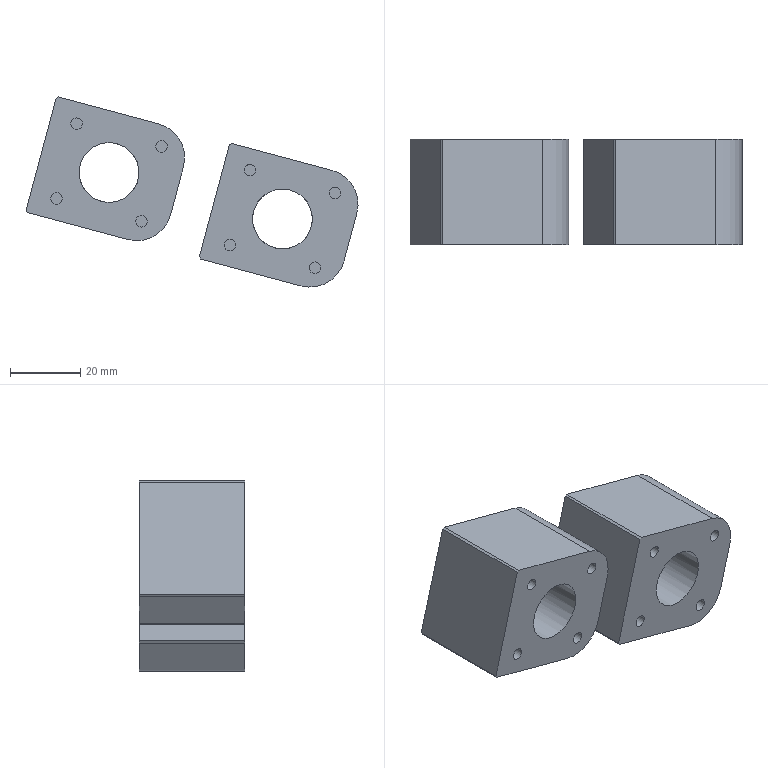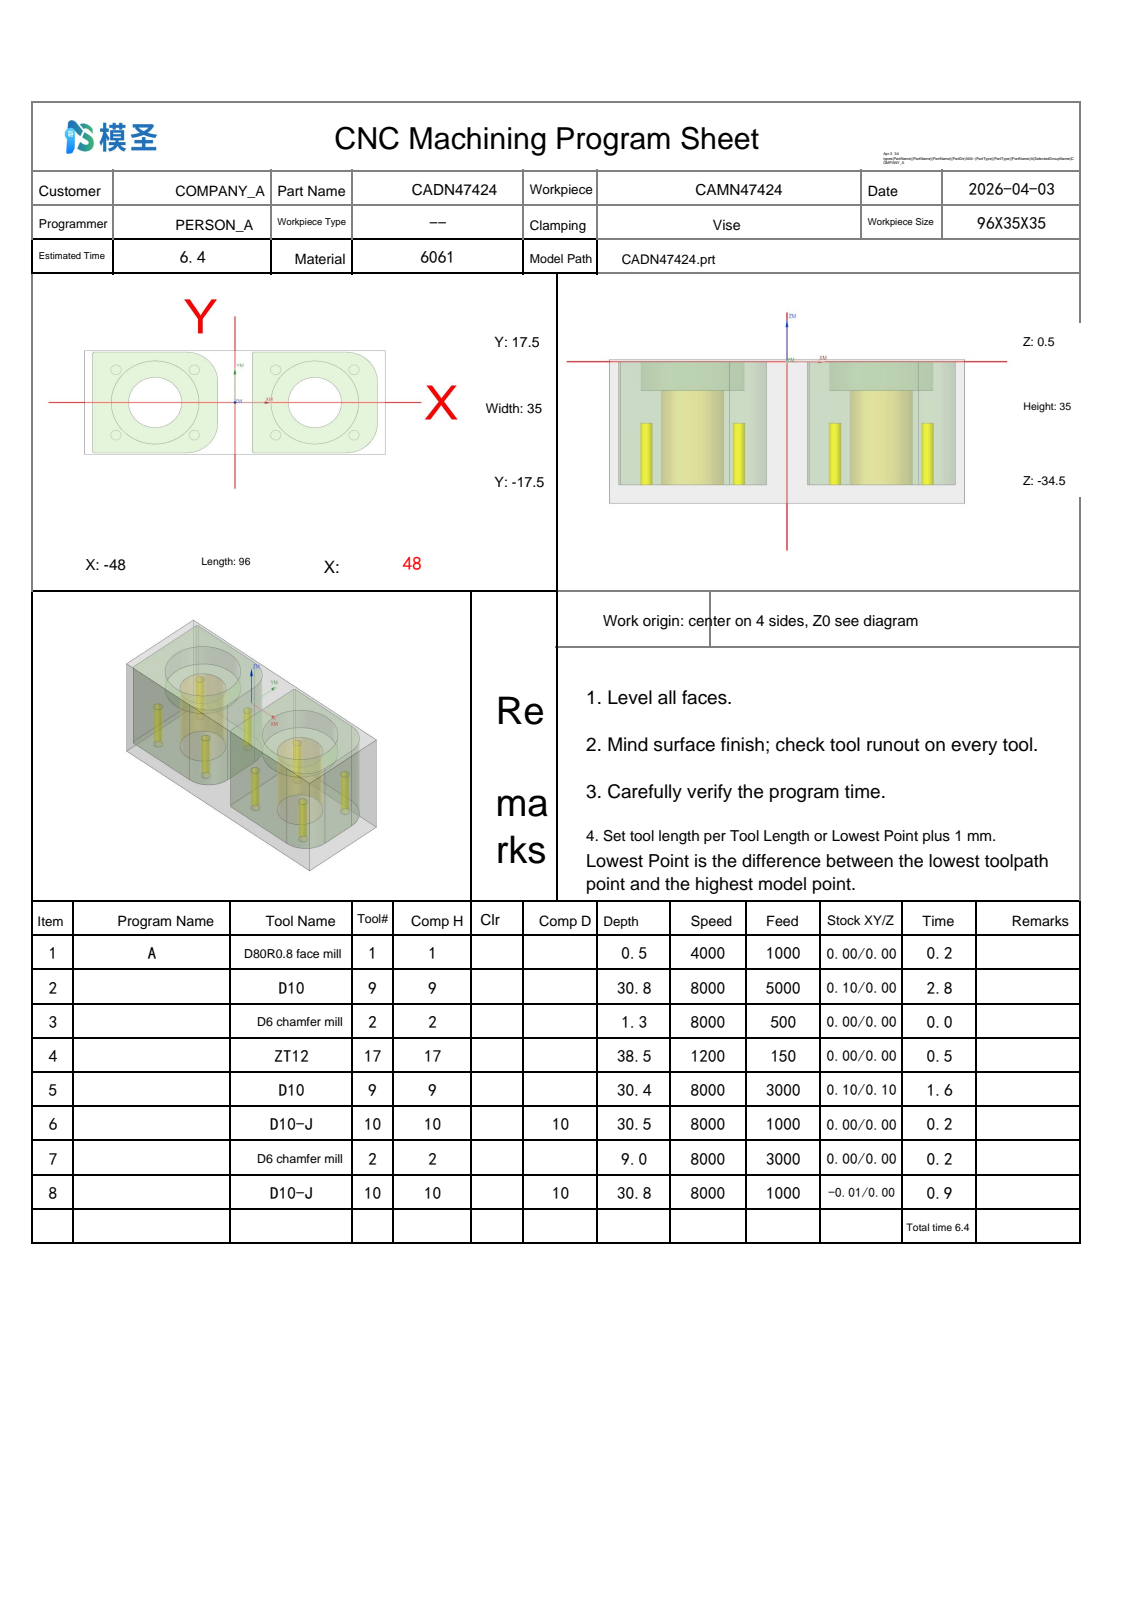NC program | NX | posted by the shop | part box 94.322 x 30 x 54.017 mm
Lines 1043 to 2047 of 2047:
N5 T09 M06
(D10  D=10. R=0. H=09 ce=0.10 di=0.10)
G00 G90 G54 X31.535 Y-6.551 M03 S8000
G43 H09 Z20.
M08
Z1.
G01 X32.075 Y-6.072 Z.962 F3000.
X33.155 Y-4.638 Z.868
X33.927 Y-3.016 Z.774
X34.306 Y-1.601 Z.697
X34.448 Y.189 Z.603
X34.23 Y1.971 Z.509
X33.661 Y3.675 Z.415
X32.763 Y5.23 Z.321
X31.572 Y6.575 Z.227
X30.138 Y7.655 Z.132
X28.516 Y8.427 Z.038
X27.809 Y8.616 Z0.0
G03 X16.884 Y2.309 Z-.123 I-2.309 J-8.616
X23.191 Y-8.616 Z-.246 I8.616 J-2.309
X34.116 Y-2.309 Z-.37 I2.309 J8.616
X27.809 Y8.616 Z-.493 I-8.616 J2.309
X16.884 Y2.309 Z-.616 I-2.309 J-8.616
X23.191 Y-8.616 Z-.739 I8.616 J-2.309
X34.116 Y-2.309 Z-.863 I2.309 J8.616
X27.809 Y8.616 Z-.986 I-8.616 J2.309
X16.884 Y2.309 Z-1.109 I-2.309 J-8.616
X23.191 Y-8.616 Z-1.232 I8.616 J-2.309
X34.116 Y-2.309 Z-1.355 I2.309 J8.616
X27.809 Y8.616 Z-1.479 I-8.616 J2.309
X16.884 Y2.309 Z-1.602 I-2.309 J-8.616
X23.191 Y-8.616 Z-1.725 I8.616 J-2.309
X34.116 Y-2.309 Z-1.848 I2.309 J8.616
X27.809 Y8.616 Z-1.971 I-8.616 J2.309
X16.884 Y2.309 Z-2.095 I-2.309 J-8.616
X23.191 Y-8.616 Z-2.218 I8.616 J-2.309
X34.116 Y-2.309 Z-2.341 I2.309 J8.616
X27.809 Y8.616 Z-2.464 I-8.616 J2.309
X16.884 Y2.309 Z-2.588 I-2.309 J-8.616
X23.191 Y-8.616 Z-2.711 I8.616 J-2.309
X34.116 Y-2.309 Z-2.834 I2.309 J8.616
X27.809 Y8.616 Z-2.957 I-8.616 J2.309
X16.884 Y2.309 Z-3.08 I-2.309 J-8.616
X23.191 Y-8.616 Z-3.204 I8.616 J-2.309
X34.116 Y-2.309 Z-3.327 I2.309 J8.616
X27.809 Y8.616 Z-3.45 I-8.616 J2.309
X16.884 Y2.309 Z-3.573 I-2.309 J-8.616
X23.191 Y-8.616 Z-3.696 I8.616 J-2.309
X34.116 Y-2.309 Z-3.82 I2.309 J8.616
X27.809 Y8.616 Z-3.943 I-8.616 J2.309
X16.884 Y2.309 Z-4.066 I-2.309 J-8.616
X23.191 Y-8.616 Z-4.189 I8.616 J-2.309
X34.116 Y-2.309 Z-4.313 I2.309 J8.616
X27.809 Y8.616 Z-4.436 I-8.616 J2.309
X16.884 Y2.309 Z-4.559 I-2.309 J-8.616
X23.191 Y-8.616 Z-4.682 I8.616 J-2.309
X34.116 Y-2.309 Z-4.805 I2.309 J8.616
X27.809 Y8.616 Z-4.929 I-8.616 J2.309
X16.884 Y2.309 Z-5.052 I-2.309 J-8.616
X23.191 Y-8.616 Z-5.175 I8.616 J-2.309
X34.116 Y-2.309 Z-5.298 I2.309 J8.616
X27.809 Y8.616 Z-5.421 I-8.616 J2.309
X16.884 Y2.309 Z-5.545 I-2.309 J-8.616
X23.191 Y-8.616 Z-5.668 I8.616 J-2.309
X34.116 Y-2.309 Z-5.791 I2.309 J8.616
X27.809 Y8.616 Z-5.914 I-8.616 J2.309
X16.884 Y2.309 Z-6.038 I-2.309 J-8.616
X23.191 Y-8.616 Z-6.161 I8.616 J-2.309
X34.116 Y-2.309 Z-6.284 I2.309 J8.616
X27.809 Y8.616 Z-6.407 I-8.616 J2.309
X16.884 Y2.309 Z-6.53 I-2.309 J-8.616
X23.191 Y-8.616 Z-6.654 I8.616 J-2.309
X34.116 Y-2.309 Z-6.777 I2.309 J8.616
X27.809 Y8.616 Z-6.9 I-8.616 J2.309
X25.5 Y8.92 I-2.309 J-8.616
X16.58 Y0.0 I0.0 J-8.92
X25.5 Y-8.92 I8.92 J0.0
X34.42 Y0.0 I0.0 J8.92
X27.809 Y8.616 I-8.92 J0.0
X27.42 Y8.711 I-2.309 J-8.616
G01 Z-5.9
G00 Z20.
X-31.535 Y6.551
Z1.
G01 X-32.075 Y6.072 Z.962
X-33.155 Y4.638 Z.868
X-33.927 Y3.016 Z.774
X-34.306 Y1.601 Z.697
X-34.448 Y-.189 Z.603
X-34.23 Y-1.971 Z.509
X-33.661 Y-3.675 Z.415
X-32.763 Y-5.23 Z.321
X-31.572 Y-6.575 Z.227
X-30.138 Y-7.655 Z.132
X-28.516 Y-8.427 Z.038
X-27.809 Y-8.616 Z0.0
G03 X-16.884 Y-2.309 Z-.123 I2.309 J8.616
X-18.483 Y5.508 Z-.196 I-8.616 J2.309
X-23.191 Y8.616 Z-.246 I-7.017 J-5.508
X-34.116 Y2.309 Z-.37 I-2.309 J-8.616
X-27.809 Y-8.616 Z-.493 I8.616 J-2.309
X-16.884 Y-2.309 Z-.616 I2.309 J8.616
X-18.483 Y5.508 Z-.689 I-8.616 J2.309
X-23.191 Y8.616 Z-.739 I-7.017 J-5.508
X-34.116 Y2.309 Z-.863 I-2.309 J-8.616
X-27.809 Y-8.616 Z-.986 I8.616 J-2.309
X-16.884 Y-2.309 Z-1.109 I2.309 J8.616
X-18.483 Y5.508 Z-1.182 I-8.616 J2.309
X-23.191 Y8.616 Z-1.232 I-7.017 J-5.508
X-34.116 Y2.309 Z-1.355 I-2.309 J-8.616
X-27.809 Y-8.616 Z-1.479 I8.616 J-2.309
X-16.884 Y-2.309 Z-1.602 I2.309 J8.616
X-18.483 Y5.508 Z-1.675 I-8.616 J2.309
X-23.191 Y8.616 Z-1.725 I-7.017 J-5.508
X-34.116 Y2.309 Z-1.848 I-2.309 J-8.616
X-27.809 Y-8.616 Z-1.971 I8.616 J-2.309
X-16.884 Y-2.309 Z-2.095 I2.309 J8.616
X-18.483 Y5.508 Z-2.167 I-8.616 J2.309
X-23.191 Y8.616 Z-2.218 I-7.017 J-5.508
X-34.116 Y2.309 Z-2.341 I-2.309 J-8.616
X-27.809 Y-8.616 Z-2.464 I8.616 J-2.309
X-16.884 Y-2.309 Z-2.588 I2.309 J8.616
X-18.483 Y5.508 Z-2.66 I-8.616 J2.309
X-23.191 Y8.616 Z-2.711 I-7.017 J-5.508
X-34.116 Y2.309 Z-2.834 I-2.309 J-8.616
X-27.809 Y-8.616 Z-2.957 I8.616 J-2.309
X-16.884 Y-2.309 Z-3.08 I2.309 J8.616
X-18.483 Y5.508 Z-3.153 I-8.616 J2.309
X-23.191 Y8.616 Z-3.204 I-7.017 J-5.508
X-34.116 Y2.309 Z-3.327 I-2.309 J-8.616
X-27.809 Y-8.616 Z-3.45 I8.616 J-2.309
X-16.884 Y-2.309 Z-3.573 I2.309 J8.616
X-18.483 Y5.508 Z-3.646 I-8.616 J2.309
X-23.191 Y8.616 Z-3.696 I-7.017 J-5.508
X-34.116 Y2.309 Z-3.82 I-2.309 J-8.616
X-27.809 Y-8.616 Z-3.943 I8.616 J-2.309
X-16.884 Y-2.309 Z-4.066 I2.309 J8.616
X-18.483 Y5.508 Z-4.139 I-8.616 J2.309
X-23.191 Y8.616 Z-4.189 I-7.017 J-5.508
X-34.116 Y2.309 Z-4.313 I-2.309 J-8.616
X-27.809 Y-8.616 Z-4.436 I8.616 J-2.309
X-16.884 Y-2.309 Z-4.559 I2.309 J8.616
X-18.483 Y5.508 Z-4.632 I-8.616 J2.309
X-23.191 Y8.616 Z-4.682 I-7.017 J-5.508
X-34.116 Y2.309 Z-4.805 I-2.309 J-8.616
X-27.809 Y-8.616 Z-4.929 I8.616 J-2.309
X-16.884 Y-2.309 Z-5.052 I2.309 J8.616
X-18.483 Y5.508 Z-5.125 I-8.616 J2.309
X-23.191 Y8.616 Z-5.175 I-7.017 J-5.508
X-34.116 Y2.309 Z-5.298 I-2.309 J-8.616
X-27.809 Y-8.616 Z-5.421 I8.616 J-2.309
X-16.884 Y-2.309 Z-5.545 I2.309 J8.616
X-18.483 Y5.508 Z-5.617 I-8.616 J2.309
X-23.191 Y8.616 Z-5.668 I-7.017 J-5.508
X-34.116 Y2.309 Z-5.791 I-2.309 J-8.616
X-27.809 Y-8.616 Z-5.914 I8.616 J-2.309
X-16.884 Y-2.309 Z-6.038 I2.309 J8.616
X-18.483 Y5.508 Z-6.11 I-8.616 J2.309
X-23.191 Y8.616 Z-6.161 I-7.017 J-5.508
X-34.116 Y2.309 Z-6.284 I-2.309 J-8.616
X-27.809 Y-8.616 Z-6.407 I8.616 J-2.309
X-16.884 Y-2.309 Z-6.53 I2.309 J8.616
X-18.483 Y5.508 Z-6.603 I-8.616 J2.309
X-23.191 Y8.616 Z-6.654 I-7.017 J-5.508
X-34.116 Y2.309 Z-6.777 I-2.309 J-8.616
X-27.809 Y-8.616 Z-6.9 I8.616 J-2.309
X-25.5 Y-8.92 I2.309 J8.616
X-16.58 Y0.0 I0.0 J8.92
X-25.5 Y8.92 I-8.92 J0.0
X-34.42 Y0.0 I0.0 J-8.92
X-27.809 Y-8.616 I8.92 J0.0
X-27.42 Y-8.711 I2.309 J8.616
G01 Z-5.9
G00 Z20.
G00 G90 X24.068 Y3.077 M03 S8000
Z20.
Z-6.
G01 X23.785 Y2.97 Z-6.016 F2000.
X22.923 Y2.263 Z-6.074
X22.333 Y1.317 Z-6.133
X22.099 Y.443 Z-6.18
X22.136 Y-.672 Z-6.239
X22.53 Y-1.715 Z-6.297
X23.237 Y-2.577 Z-6.355
X24.183 Y-3.167 Z-6.414
X25.057 Y-3.401 Z-6.461
X26.172 Y-3.364 Z-6.52
X27.215 Y-2.97 Z-6.578
X28.077 Y-2.263 Z-6.637
X28.667 Y-1.317 Z-6.695
X28.901 Y-.443 Z-6.743
X28.864 Y.672 Z-6.801
X28.47 Y1.715 Z-6.859
X27.763 Y2.577 Z-6.918
X26.817 Y3.167 Z-6.976
X26.38 Y3.284 Z-7.
G03 X22.216 Y.88 Z-7.124 I-.88 J-3.284
X24.62 Y-3.284 Z-7.249 I3.284 J-.88
X28.784 Y-.88 Z-7.373 I.88 J3.284
X26.38 Y3.284 Z-7.498 I-3.284 J.88
X22.216 Y.88 Z-7.622 I-.88 J-3.284
X24.62 Y-3.284 Z-7.747 I3.284 J-.88
X28.784 Y-.88 Z-7.871 I.88 J3.284
X26.38 Y3.284 Z-7.996 I-3.284 J.88
X22.216 Y.88 Z-8.12 I-.88 J-3.284
X24.62 Y-3.284 Z-8.245 I3.284 J-.88
X28.784 Y-.88 Z-8.369 I.88 J3.284
X26.38 Y3.284 Z-8.493 I-3.284 J.88
X22.216 Y.88 Z-8.618 I-.88 J-3.284
X24.62 Y-3.284 Z-8.742 I3.284 J-.88
X28.784 Y-.88 Z-8.867 I.88 J3.284
X26.38 Y3.284 Z-8.991 I-3.284 J.88
X22.216 Y.88 Z-9.116 I-.88 J-3.284
X24.62 Y-3.284 Z-9.24 I3.284 J-.88
X28.784 Y-.88 Z-9.365 I.88 J3.284
X26.38 Y3.284 Z-9.489 I-3.284 J.88
X22.216 Y.88 Z-9.614 I-.88 J-3.284
X24.62 Y-3.284 Z-9.738 I3.284 J-.88
X28.784 Y-.88 Z-9.863 I.88 J3.284
X26.38 Y3.284 Z-9.987 I-3.284 J.88
X22.216 Y.88 Z-10.111 I-.88 J-3.284
X24.62 Y-3.284 Z-10.236 I3.284 J-.88
X28.784 Y-.88 Z-10.36 I.88 J3.284
X26.38 Y3.284 Z-10.485 I-3.284 J.88
X22.216 Y.88 Z-10.609 I-.88 J-3.284
X24.62 Y-3.284 Z-10.734 I3.284 J-.88
X28.784 Y-.88 Z-10.858 I.88 J3.284
X26.38 Y3.284 Z-10.983 I-3.284 J.88
X22.216 Y.88 Z-11.107 I-.88 J-3.284
X24.62 Y-3.284 Z-11.232 I3.284 J-.88
X28.784 Y-.88 Z-11.356 I.88 J3.284
X26.38 Y3.284 Z-11.48 I-3.284 J.88
X22.216 Y.88 Z-11.605 I-.88 J-3.284
X24.62 Y-3.284 Z-11.729 I3.284 J-.88
X28.784 Y-.88 Z-11.854 I.88 J3.284
X26.38 Y3.284 Z-11.978 I-3.284 J.88
X22.216 Y.88 Z-12.103 I-.88 J-3.284
X24.62 Y-3.284 Z-12.227 I3.284 J-.88
X28.784 Y-.88 Z-12.352 I.88 J3.284
X26.38 Y3.284 Z-12.476 I-3.284 J.88
X22.216 Y.88 Z-12.601 I-.88 J-3.284
X24.62 Y-3.284 Z-12.725 I3.284 J-.88
X28.784 Y-.88 Z-12.849 I.88 J3.284
X26.38 Y3.284 Z-12.974 I-3.284 J.88
X22.216 Y.88 Z-13.098 I-.88 J-3.284
X24.62 Y-3.284 Z-13.223 I3.284 J-.88
X28.784 Y-.88 Z-13.347 I.88 J3.284
X26.38 Y3.284 Z-13.472 I-3.284 J.88
X22.216 Y.88 Z-13.596 I-.88 J-3.284
X24.62 Y-3.284 Z-13.721 I3.284 J-.88
X28.784 Y-.88 Z-13.845 I.88 J3.284
X26.38 Y3.284 Z-13.97 I-3.284 J.88
X22.216 Y.88 Z-14.094 I-.88 J-3.284
X24.62 Y-3.284 Z-14.218 I3.284 J-.88
X28.784 Y-.88 Z-14.343 I.88 J3.284
X26.38 Y3.284 Z-14.467 I-3.284 J.88
X22.216 Y.88 Z-14.592 I-.88 J-3.284
X24.62 Y-3.284 Z-14.716 I3.284 J-.88
X28.784 Y-.88 Z-14.841 I.88 J3.284
X26.38 Y3.284 Z-14.965 I-3.284 J.88
X22.216 Y.88 Z-15.09 I-.88 J-3.284
X24.62 Y-3.284 Z-15.214 I3.284 J-.88
X28.784 Y-.88 Z-15.339 I.88 J3.284
X26.38 Y3.284 Z-15.463 I-3.284 J.88
X22.216 Y.88 Z-15.588 I-.88 J-3.284
X24.62 Y-3.284 Z-15.712 I3.284 J-.88
X28.784 Y-.88 Z-15.836 I.88 J3.284
X26.38 Y3.284 Z-15.961 I-3.284 J.88
X22.216 Y.88 Z-16.085 I-.88 J-3.284
X24.62 Y-3.284 Z-16.21 I3.284 J-.88
X28.784 Y-.88 Z-16.334 I.88 J3.284
X26.38 Y3.284 Z-16.459 I-3.284 J.88
X22.216 Y.88 Z-16.583 I-.88 J-3.284
X24.62 Y-3.284 Z-16.708 I3.284 J-.88
X28.784 Y-.88 Z-16.832 I.88 J3.284
X26.38 Y3.284 Z-16.957 I-3.284 J.88
X22.216 Y.88 Z-17.081 I-.88 J-3.284
X24.62 Y-3.284 Z-17.205 I3.284 J-.88
X28.784 Y-.88 Z-17.33 I.88 J3.284
X26.38 Y3.284 Z-17.454 I-3.284 J.88
X22.216 Y.88 Z-17.579 I-.88 J-3.284
X24.62 Y-3.284 Z-17.703 I3.284 J-.88
X28.784 Y-.88 Z-17.828 I.88 J3.284
X26.38 Y3.284 Z-17.952 I-3.284 J.88
X22.216 Y.88 Z-18.077 I-.88 J-3.284
X24.62 Y-3.284 Z-18.201 I3.284 J-.88
X28.784 Y-.88 Z-18.326 I.88 J3.284
X26.38 Y3.284 Z-18.45 I-3.284 J.88
X22.216 Y.88 Z-18.574 I-.88 J-3.284
X24.62 Y-3.284 Z-18.699 I3.284 J-.88
X28.784 Y-.88 Z-18.823 I.88 J3.284
X26.38 Y3.284 Z-18.948 I-3.284 J.88
X22.216 Y.88 Z-19.072 I-.88 J-3.284
X24.62 Y-3.284 Z-19.197 I3.284 J-.88
X28.784 Y-.88 Z-19.321 I.88 J3.284
X26.38 Y3.284 Z-19.446 I-3.284 J.88
X22.216 Y.88 Z-19.57 I-.88 J-3.284
X24.62 Y-3.284 Z-19.695 I3.284 J-.88
X28.784 Y-.88 Z-19.819 I.88 J3.284
X26.38 Y3.284 Z-19.943 I-3.284 J.88
X22.216 Y.88 Z-20.068 I-.88 J-3.284
X24.62 Y-3.284 Z-20.192 I3.284 J-.88
X28.784 Y-.88 Z-20.317 I.88 J3.284
X26.38 Y3.284 Z-20.441 I-3.284 J.88
X22.216 Y.88 Z-20.566 I-.88 J-3.284
X24.62 Y-3.284 Z-20.69 I3.284 J-.88
X28.784 Y-.88 Z-20.815 I.88 J3.284
X26.38 Y3.284 Z-20.939 I-3.284 J.88
X22.216 Y.88 Z-21.064 I-.88 J-3.284
X24.62 Y-3.284 Z-21.188 I3.284 J-.88
X28.784 Y-.88 Z-21.313 I.88 J3.284
X26.38 Y3.284 Z-21.437 I-3.284 J.88
X22.216 Y.88 Z-21.561 I-.88 J-3.284
X24.62 Y-3.284 Z-21.686 I3.284 J-.88
X28.784 Y-.88 Z-21.81 I.88 J3.284
X26.38 Y3.284 Z-21.935 I-3.284 J.88
X22.216 Y.88 Z-22.059 I-.88 J-3.284
X24.62 Y-3.284 Z-22.184 I3.284 J-.88
X28.784 Y-.88 Z-22.308 I.88 J3.284
X26.38 Y3.284 Z-22.433 I-3.284 J.88
X22.216 Y.88 Z-22.557 I-.88 J-3.284
X24.62 Y-3.284 Z-22.682 I3.284 J-.88
X28.784 Y-.88 Z-22.806 I.88 J3.284
X26.38 Y3.284 Z-22.93 I-3.284 J.88
X22.216 Y.88 Z-23.055 I-.88 J-3.284
X24.62 Y-3.284 Z-23.179 I3.284 J-.88
X28.784 Y-.88 Z-23.304 I.88 J3.284
X26.38 Y3.284 Z-23.428 I-3.284 J.88
X22.216 Y.88 Z-23.553 I-.88 J-3.284
X24.62 Y-3.284 Z-23.677 I3.284 J-.88
X28.784 Y-.88 Z-23.802 I.88 J3.284
X26.38 Y3.284 Z-23.926 I-3.284 J.88
X22.216 Y.88 Z-24.051 I-.88 J-3.284
X24.62 Y-3.284 Z-24.175 I3.284 J-.88
X28.784 Y-.88 Z-24.299 I.88 J3.284
X26.38 Y3.284 Z-24.424 I-3.284 J.88
X22.216 Y.88 Z-24.548 I-.88 J-3.284
X24.62 Y-3.284 Z-24.673 I3.284 J-.88
X28.784 Y-.88 Z-24.797 I.88 J3.284
X26.38 Y3.284 Z-24.922 I-3.284 J.88
X22.216 Y.88 Z-25.046 I-.88 J-3.284
X24.62 Y-3.284 Z-25.171 I3.284 J-.88
X28.784 Y-.88 Z-25.295 I.88 J3.284
X26.38 Y3.284 Z-25.42 I-3.284 J.88
X22.216 Y.88 Z-25.544 I-.88 J-3.284
X24.62 Y-3.284 Z-25.668 I3.284 J-.88
X28.784 Y-.88 Z-25.793 I.88 J3.284
X26.38 Y3.284 Z-25.917 I-3.284 J.88
X22.216 Y.88 Z-26.042 I-.88 J-3.284
X24.62 Y-3.284 Z-26.166 I3.284 J-.88
X28.784 Y-.88 Z-26.291 I.88 J3.284
X26.38 Y3.284 Z-26.415 I-3.284 J.88
X22.216 Y.88 Z-26.54 I-.88 J-3.284
X24.62 Y-3.284 Z-26.664 I3.284 J-.88
X28.784 Y-.88 Z-26.789 I.88 J3.284
X26.38 Y3.284 Z-26.913 I-3.284 J.88
X22.216 Y.88 Z-27.038 I-.88 J-3.284
X24.62 Y-3.284 Z-27.162 I3.284 J-.88
X28.784 Y-.88 Z-27.286 I.88 J3.284
X26.38 Y3.284 Z-27.411 I-3.284 J.88
X22.216 Y.88 Z-27.535 I-.88 J-3.284
X24.62 Y-3.284 Z-27.66 I3.284 J-.88
X28.784 Y-.88 Z-27.784 I.88 J3.284
X26.38 Y3.284 Z-27.909 I-3.284 J.88
X22.216 Y.88 Z-28.033 I-.88 J-3.284
X24.62 Y-3.284 Z-28.158 I3.284 J-.88
X28.784 Y-.88 Z-28.282 I.88 J3.284
X26.38 Y3.284 Z-28.407 I-3.284 J.88
X22.216 Y.88 Z-28.531 I-.88 J-3.284
X24.62 Y-3.284 Z-28.655 I3.284 J-.88
X28.784 Y-.88 Z-28.78 I.88 J3.284
X26.38 Y3.284 Z-28.904 I-3.284 J.88
X22.216 Y.88 Z-29.029 I-.88 J-3.284
X24.62 Y-3.284 Z-29.153 I3.284 J-.88
X28.784 Y-.88 Z-29.278 I.88 J3.284
X26.38 Y3.284 Z-29.402 I-3.284 J.88
X22.216 Y.88 Z-29.527 I-.88 J-3.284
X24.62 Y-3.284 Z-29.651 I3.284 J-.88
X28.784 Y-.88 Z-29.776 I.88 J3.284
X26.38 Y3.284 Z-29.9 I-3.284 J.88
X25.5 Y3.4 I-.88 J-3.284
X22.1 Y0.0 I0.0 J-3.4
X25.5 Y-3.4 I3.4 J0.0
X28.9 Y0.0 I0.0 J3.4
X26.38 Y3.284 I-3.4 J0.0
X25.988 Y3.365 I-.88 J-3.284
G01 Z-28.9
G00 Z20.
X-24.068 Y-3.077
Z-6.
G01 X-23.785 Y-2.97 Z-6.016
X-22.923 Y-2.263 Z-6.074
X-22.333 Y-1.317 Z-6.133
X-22.099 Y-.443 Z-6.18
X-22.136 Y.672 Z-6.239
X-22.53 Y1.715 Z-6.297
X-23.237 Y2.577 Z-6.355
X-24.183 Y3.167 Z-6.414
X-25.057 Y3.401 Z-6.461
X-26.172 Y3.364 Z-6.52
X-27.215 Y2.97 Z-6.578
X-28.077 Y2.263 Z-6.637
X-28.667 Y1.317 Z-6.695
X-28.901 Y.443 Z-6.743
X-28.864 Y-.672 Z-6.801
X-28.47 Y-1.715 Z-6.859
X-27.763 Y-2.577 Z-6.918
X-26.817 Y-3.167 Z-6.976
X-26.38 Y-3.284 Z-7.
G03 X-22.216 Y-.88 Z-7.124 I.88 J3.284
X-24.62 Y3.284 Z-7.249 I-3.284 J.88
X-28.784 Y.88 Z-7.373 I-.88 J-3.284
X-26.38 Y-3.284 Z-7.498 I3.284 J-.88
X-22.216 Y-.88 Z-7.622 I.88 J3.284
X-24.62 Y3.284 Z-7.747 I-3.284 J.88
X-28.784 Y.88 Z-7.871 I-.88 J-3.284
X-26.38 Y-3.284 Z-7.996 I3.284 J-.88
X-22.216 Y-.88 Z-8.12 I.88 J3.284
X-24.62 Y3.284 Z-8.245 I-3.284 J.88
X-28.784 Y.88 Z-8.369 I-.88 J-3.284
X-26.38 Y-3.284 Z-8.493 I3.284 J-.88
X-22.216 Y-.88 Z-8.618 I.88 J3.284
X-24.62 Y3.284 Z-8.742 I-3.284 J.88
X-28.784 Y.88 Z-8.867 I-.88 J-3.284
X-26.38 Y-3.284 Z-8.991 I3.284 J-.88
X-22.216 Y-.88 Z-9.116 I.88 J3.284
X-24.62 Y3.284 Z-9.24 I-3.284 J.88
X-28.784 Y.88 Z-9.365 I-.88 J-3.284
X-26.38 Y-3.284 Z-9.489 I3.284 J-.88
X-22.216 Y-.88 Z-9.614 I.88 J3.284
X-24.62 Y3.284 Z-9.738 I-3.284 J.88
X-28.784 Y.88 Z-9.863 I-.88 J-3.284
X-26.38 Y-3.284 Z-9.987 I3.284 J-.88
X-22.216 Y-.88 Z-10.111 I.88 J3.284
X-24.62 Y3.284 Z-10.236 I-3.284 J.88
X-28.784 Y.88 Z-10.36 I-.88 J-3.284
X-26.38 Y-3.284 Z-10.485 I3.284 J-.88
X-22.216 Y-.88 Z-10.609 I.88 J3.284
X-24.62 Y3.284 Z-10.734 I-3.284 J.88
X-28.784 Y.88 Z-10.858 I-.88 J-3.284
X-26.38 Y-3.284 Z-10.983 I3.284 J-.88
X-22.216 Y-.88 Z-11.107 I.88 J3.284
X-24.62 Y3.284 Z-11.232 I-3.284 J.88
X-28.784 Y.88 Z-11.356 I-.88 J-3.284
X-26.38 Y-3.284 Z-11.48 I3.284 J-.88
X-22.216 Y-.88 Z-11.605 I.88 J3.284
X-24.62 Y3.284 Z-11.729 I-3.284 J.88
X-28.784 Y.88 Z-11.854 I-.88 J-3.284
X-26.38 Y-3.284 Z-11.978 I3.284 J-.88
X-22.216 Y-.88 Z-12.103 I.88 J3.284
X-24.62 Y3.284 Z-12.227 I-3.284 J.88
X-28.784 Y.88 Z-12.352 I-.88 J-3.284
X-26.38 Y-3.284 Z-12.476 I3.284 J-.88
X-22.216 Y-.88 Z-12.601 I.88 J3.284
X-24.62 Y3.284 Z-12.725 I-3.284 J.88
X-28.784 Y.88 Z-12.849 I-.88 J-3.284
X-26.38 Y-3.284 Z-12.974 I3.284 J-.88
X-22.216 Y-.88 Z-13.098 I.88 J3.284
X-24.62 Y3.284 Z-13.223 I-3.284 J.88
X-28.784 Y.88 Z-13.347 I-.88 J-3.284
X-26.38 Y-3.284 Z-13.472 I3.284 J-.88
X-22.216 Y-.88 Z-13.596 I.88 J3.284
X-24.62 Y3.284 Z-13.721 I-3.284 J.88
X-28.784 Y.88 Z-13.845 I-.88 J-3.284
X-26.38 Y-3.284 Z-13.97 I3.284 J-.88
X-22.216 Y-.88 Z-14.094 I.88 J3.284
X-24.62 Y3.284 Z-14.218 I-3.284 J.88
X-28.784 Y.88 Z-14.343 I-.88 J-3.284
X-26.38 Y-3.284 Z-14.467 I3.284 J-.88
X-22.216 Y-.88 Z-14.592 I.88 J3.284
X-24.62 Y3.284 Z-14.716 I-3.284 J.88
X-28.784 Y.88 Z-14.841 I-.88 J-3.284
X-26.38 Y-3.284 Z-14.965 I3.284 J-.88
X-22.216 Y-.88 Z-15.09 I.88 J3.284
X-24.62 Y3.284 Z-15.214 I-3.284 J.88
X-28.784 Y.88 Z-15.339 I-.88 J-3.284
X-26.38 Y-3.284 Z-15.463 I3.284 J-.88
X-22.216 Y-.88 Z-15.588 I.88 J3.284
X-24.62 Y3.284 Z-15.712 I-3.284 J.88
X-28.784 Y.88 Z-15.836 I-.88 J-3.284
X-26.38 Y-3.284 Z-15.961 I3.284 J-.88
X-22.216 Y-.88 Z-16.085 I.88 J3.284
X-24.62 Y3.284 Z-16.21 I-3.284 J.88
X-28.784 Y.88 Z-16.334 I-.88 J-3.284
X-26.38 Y-3.284 Z-16.459 I3.284 J-.88
X-22.216 Y-.88 Z-16.583 I.88 J3.284
X-24.62 Y3.284 Z-16.708 I-3.284 J.88
X-28.784 Y.88 Z-16.832 I-.88 J-3.284
X-26.38 Y-3.284 Z-16.957 I3.284 J-.88
X-22.216 Y-.88 Z-17.081 I.88 J3.284
X-24.62 Y3.284 Z-17.205 I-3.284 J.88
X-28.784 Y.88 Z-17.33 I-.88 J-3.284
X-26.38 Y-3.284 Z-17.454 I3.284 J-.88
X-22.216 Y-.88 Z-17.579 I.88 J3.284
X-24.62 Y3.284 Z-17.703 I-3.284 J.88
X-28.784 Y.88 Z-17.828 I-.88 J-3.284
X-26.38 Y-3.284 Z-17.952 I3.284 J-.88
X-22.216 Y-.88 Z-18.077 I.88 J3.284
X-24.62 Y3.284 Z-18.201 I-3.284 J.88
X-28.784 Y.88 Z-18.326 I-.88 J-3.284
X-26.38 Y-3.284 Z-18.45 I3.284 J-.88
X-22.216 Y-.88 Z-18.574 I.88 J3.284
X-24.62 Y3.284 Z-18.699 I-3.284 J.88
X-28.784 Y.88 Z-18.823 I-.88 J-3.284
X-26.38 Y-3.284 Z-18.948 I3.284 J-.88
X-22.216 Y-.88 Z-19.072 I.88 J3.284
X-24.62 Y3.284 Z-19.197 I-3.284 J.88
X-28.784 Y.88 Z-19.321 I-.88 J-3.284
X-26.38 Y-3.284 Z-19.446 I3.284 J-.88
X-22.216 Y-.88 Z-19.57 I.88 J3.284
X-24.62 Y3.284 Z-19.695 I-3.284 J.88
X-28.784 Y.88 Z-19.819 I-.88 J-3.284
X-26.38 Y-3.284 Z-19.943 I3.284 J-.88
X-22.216 Y-.88 Z-20.068 I.88 J3.284
X-24.62 Y3.284 Z-20.192 I-3.284 J.88
X-28.784 Y.88 Z-20.317 I-.88 J-3.284
X-26.38 Y-3.284 Z-20.441 I3.284 J-.88
X-22.216 Y-.88 Z-20.566 I.88 J3.284
X-24.62 Y3.284 Z-20.69 I-3.284 J.88
X-28.784 Y.88 Z-20.815 I-.88 J-3.284
X-26.38 Y-3.284 Z-20.939 I3.284 J-.88
X-22.216 Y-.88 Z-21.064 I.88 J3.284
X-24.62 Y3.284 Z-21.188 I-3.284 J.88
X-28.784 Y.88 Z-21.313 I-.88 J-3.284
X-26.38 Y-3.284 Z-21.437 I3.284 J-.88
X-22.216 Y-.88 Z-21.561 I.88 J3.284
X-24.62 Y3.284 Z-21.686 I-3.284 J.88
X-28.784 Y.88 Z-21.81 I-.88 J-3.284
X-26.38 Y-3.284 Z-21.935 I3.284 J-.88
X-22.216 Y-.88 Z-22.059 I.88 J3.284
X-24.62 Y3.284 Z-22.184 I-3.284 J.88
X-28.784 Y.88 Z-22.308 I-.88 J-3.284
X-26.38 Y-3.284 Z-22.433 I3.284 J-.88
X-22.216 Y-.88 Z-22.557 I.88 J3.284
X-24.62 Y3.284 Z-22.682 I-3.284 J.88
X-28.784 Y.88 Z-22.806 I-.88 J-3.284
X-26.38 Y-3.284 Z-22.93 I3.284 J-.88
X-22.216 Y-.88 Z-23.055 I.88 J3.284
X-24.62 Y3.284 Z-23.179 I-3.284 J.88
X-28.784 Y.88 Z-23.304 I-.88 J-3.284
X-26.38 Y-3.284 Z-23.428 I3.284 J-.88
X-22.216 Y-.88 Z-23.553 I.88 J3.284
X-24.62 Y3.284 Z-23.677 I-3.284 J.88
X-28.784 Y.88 Z-23.802 I-.88 J-3.284
X-26.38 Y-3.284 Z-23.926 I3.284 J-.88
X-22.216 Y-.88 Z-24.051 I.88 J3.284
X-24.62 Y3.284 Z-24.175 I-3.284 J.88
X-28.784 Y.88 Z-24.299 I-.88 J-3.284
X-26.38 Y-3.284 Z-24.424 I3.284 J-.88
X-22.216 Y-.88 Z-24.548 I.88 J3.284
X-24.62 Y3.284 Z-24.673 I-3.284 J.88
X-28.784 Y.88 Z-24.797 I-.88 J-3.284
X-26.38 Y-3.284 Z-24.922 I3.284 J-.88
X-22.216 Y-.88 Z-25.046 I.88 J3.284
X-24.62 Y3.284 Z-25.171 I-3.284 J.88
X-28.784 Y.88 Z-25.295 I-.88 J-3.284
X-26.38 Y-3.284 Z-25.42 I3.284 J-.88
X-22.216 Y-.88 Z-25.544 I.88 J3.284
X-24.62 Y3.284 Z-25.668 I-3.284 J.88
X-28.784 Y.88 Z-25.793 I-.88 J-3.284
X-26.38 Y-3.284 Z-25.917 I3.284 J-.88
X-22.216 Y-.88 Z-26.042 I.88 J3.284
X-24.62 Y3.284 Z-26.166 I-3.284 J.88
X-28.784 Y.88 Z-26.291 I-.88 J-3.284
X-26.38 Y-3.284 Z-26.415 I3.284 J-.88
X-22.216 Y-.88 Z-26.54 I.88 J3.284
X-24.62 Y3.284 Z-26.664 I-3.284 J.88
X-28.784 Y.88 Z-26.789 I-.88 J-3.284
X-26.38 Y-3.284 Z-26.913 I3.284 J-.88
X-22.216 Y-.88 Z-27.038 I.88 J3.284
X-24.62 Y3.284 Z-27.162 I-3.284 J.88
X-28.784 Y.88 Z-27.286 I-.88 J-3.284
X-26.38 Y-3.284 Z-27.411 I3.284 J-.88
X-22.216 Y-.88 Z-27.535 I.88 J3.284
X-24.62 Y3.284 Z-27.66 I-3.284 J.88
X-28.784 Y.88 Z-27.784 I-.88 J-3.284
X-26.38 Y-3.284 Z-27.909 I3.284 J-.88
X-22.216 Y-.88 Z-28.033 I.88 J3.284
X-24.62 Y3.284 Z-28.158 I-3.284 J.88
X-28.784 Y.88 Z-28.282 I-.88 J-3.284
X-26.38 Y-3.284 Z-28.407 I3.284 J-.88
X-22.216 Y-.88 Z-28.531 I.88 J3.284
X-24.62 Y3.284 Z-28.655 I-3.284 J.88
X-28.784 Y.88 Z-28.78 I-.88 J-3.284
X-26.38 Y-3.284 Z-28.904 I3.284 J-.88
X-22.216 Y-.88 Z-29.029 I.88 J3.284
X-24.62 Y3.284 Z-29.153 I-3.284 J.88
X-28.784 Y.88 Z-29.278 I-.88 J-3.284
X-26.38 Y-3.284 Z-29.402 I3.284 J-.88
X-22.216 Y-.88 Z-29.527 I.88 J3.284
X-24.62 Y3.284 Z-29.651 I-3.284 J.88
X-28.784 Y.88 Z-29.776 I-.88 J-3.284
X-26.38 Y-3.284 Z-29.9 I3.284 J-.88
X-25.5 Y-3.4 I.88 J3.284
X-22.1 Y0.0 I0.0 J3.4
X-25.5 Y3.4 I-3.4 J0.0
X-28.9 Y0.0 I0.0 J-3.4
X-26.38 Y-3.284 I3.4 J0.0
X-25.988 Y-3.365 I.88 J3.284
G01 Z-28.9
G00 Z20.
G91 G28 Z0.0
M05
M09
G91 G28 Z0.0
M01
N6 T10 M06
(D10-J  D=10. R=0. H=10 ce=0.00 di=0.00)
G00 G90 G54 X27.24 Y.696 M03 S8000
G43 H10 Z10.5
M08
Z-13.167
G01 Z-14.667 F1000.
G41 D10
X27.467 Y1.544
G03 X27.518 Y1.932 I-1.449 J.388
X26.406 Y3.381 I-1.5 J0.0
X25.5 Y3.5 I-.906 J-3.381
X22. Y0.0 I0.0 J-3.5
X25.5 Y-3.5 I3.5 J0.0
X29. Y0.0 I0.0 J3.5
X26.406 Y3.381 I-3.5 J0.0
X26.014 Y3.462 I-.906 J-3.381
X25.794 Y3.478 I-.22 J-1.484
X24.31 Y2.199 I0.0 J-1.5
G01 X24.211 Y1.529
G40 X24.181 Y1.331
Z-13.167
G00 X27.24 Y.696
Z-20.833
G01 Z-22.333
G41 D10
X27.467 Y1.544
G03 X27.518 Y1.932 I-1.449 J.388
X26.406 Y3.381 I-1.5 J0.0
X25.5 Y3.5 I-.906 J-3.381
X22. Y0.0 I0.0 J-3.5
X25.5 Y-3.5 I3.5 J0.0
X29. Y0.0 I0.0 J3.5
X26.406 Y3.381 I-3.5 J0.0
X26.014 Y3.462 I-.906 J-3.381
X25.794 Y3.478 I-.22 J-1.484
X24.31 Y2.199 I0.0 J-1.5
G01 X24.211 Y1.529
G40 X24.181 Y1.331
Z-20.833
G00 X27.24 Y.696
Z-28.5
G01 Z-30.
G41 D10
X27.467 Y1.544
G03 X27.518 Y1.932 I-1.449 J.388
X26.406 Y3.381 I-1.5 J0.0
X25.5 Y3.5 I-.906 J-3.381
X22. Y0.0 I0.0 J-3.5
X25.5 Y-3.5 I3.5 J0.0
X29. Y0.0 I0.0 J3.5
X26.406 Y3.381 I-3.5 J0.0
X26.014 Y3.462 I-.906 J-3.381
X25.794 Y3.478 I-.22 J-1.484
X24.31 Y2.199 I0.0 J-1.5
G01 X24.211 Y1.529
G40 X24.181 Y1.331
Z-28.5
G00 Z10.5
X-27.24 Y-.696
Z-13.167
G01 Z-14.667
G41 D10
X-27.467 Y-1.544
G03 X-27.518 Y-1.932 I1.449 J-.388
X-26.406 Y-3.381 I1.5 J0.0
X-25.5 Y-3.5 I.906 J3.381
X-22. Y0.0 I0.0 J3.5
X-25.5 Y3.5 I-3.5 J0.0
X-29. Y0.0 I0.0 J-3.5
X-26.406 Y-3.381 I3.5 J0.0
X-26.014 Y-3.462 I.906 J3.381
X-25.794 Y-3.478 I.22 J1.484
X-24.31 Y-2.199 I0.0 J1.5
G01 X-24.211 Y-1.529
G40 X-24.181 Y-1.331
Z-13.167
G00 X-27.24 Y-.696
Z-20.833
G01 Z-22.333
G41 D10
X-27.467 Y-1.544
G03 X-27.518 Y-1.932 I1.449 J-.388
X-26.406 Y-3.381 I1.5 J0.0
X-25.5 Y-3.5 I.906 J3.381
X-22. Y0.0 I0.0 J3.5
X-25.5 Y3.5 I-3.5 J0.0
X-29. Y0.0 I0.0 J-3.5
X-26.406 Y-3.381 I3.5 J0.0
X-26.014 Y-3.462 I.906 J3.381
X-25.794 Y-3.478 I.22 J1.484
X-24.31 Y-2.199 I0.0 J1.5
G01 X-24.211 Y-1.529
G40 X-24.181 Y-1.331
Z-20.833
G00 X-27.24 Y-.696
Z-28.5
G01 Z-30.
G41 D10
X-27.467 Y-1.544
G03 X-27.518 Y-1.932 I1.449 J-.388
X-26.406 Y-3.381 I1.5 J0.0
X-25.5 Y-3.5 I.906 J3.381
X-22. Y0.0 I0.0 J3.5
X-25.5 Y3.5 I-3.5 J0.0
X-29. Y0.0 I0.0 J-3.5
X-26.406 Y-3.381 I3.5 J0.0
X-26.014 Y-3.462 I.906 J3.381
X-25.794 Y-3.478 I.22 J1.484
X-24.31 Y-2.199 I0.0 J1.5
G01 X-24.211 Y-1.529
G40 X-24.181 Y-1.331
Z-28.5
G00 Z10.5
G91 G28 Z0.0
M05
M09
G91 G28 Z0.0
M01
N7 T02 M06
(D6 chamfer mill  D=6. R=0. H=02 ce=0.00 di=0.00)
G00 G90 G54 X-47.328 Y-.25 M03 S8000
G43 H02 Z20.
M08
Z2.399
G01 Z-1.499 F3000.
G03 X-47.028 Y-.33 I.3 J.52
X-46.508 Y-.03 I0.0 J.6
G01 X-46.5 Y0.0
Y16.5
X-46.466 Y16.759
X-46.366 Y17.
X-46.207 Y17.207
X-45.707 Y17.707
X-45.5 Y17.866
X-45.259 Y17.966
X-45. Y18.
X-15.5
G02 X-4.5 Y7. I0.0 J-11.
G01 Y-7.
G02 X-15.5 Y-18. I-11. J0.0
G01 X-45.
X-45.259 Y-17.966
X-45.5 Y-17.866
X-45.707 Y-17.707
X-46.207 Y-17.207
X-46.366 Y-17.
X-46.466 Y-16.759
X-46.5 Y-16.5
Y0.0
X-46.508 Y.03
G03 X-47.028 Y.33 I-.52 J-.3
X-47.328 Y.25 I0.0 J-.6
G01 Z2.399
G00 Z20.
X-28.929 Y-11.714
Z2.419
G01 Z-1.499
G03 X-29.089 Y-12.122 I.44 J-.408
X-28.897 Y-12.562 I.6 J0.0
G01 X-28.87 Y-12.576
G03 X-25.5 Y-13.02 I3.37 J12.576
X-12.48 Y0.0 I0.0 J13.02
X-25.5 Y13.02 I-13.02 J0.0
X-38.52 Y0.0 I0.0 J-13.02
X-28.87 Y-12.576 I13.02 J0.0
G01 X-28.839 Y-12.578
G03 X-28.372 Y-11.993 I-.134 J.585
G01 X-28.387 Y-11.859
Z2.419
G00 Z20.
X20.5 Y18.828
Z2.399
G01 Z-1.499
G03 X20.42 Y18.528 I.52 J-.3
X20.72 Y18.008 I.6 J0.0
G01 X20.75 Y18.
X35.5
G02 X46.5 Y7. I0.0 J-11.
G01 Y-7.
G02 X35.5 Y-18. I-11. J0.0
G01 X6.
X5.741 Y-17.966
X5.5 Y-17.866
X5.293 Y-17.707
X4.793 Y-17.207
X4.634 Y-17.
X4.534 Y-16.759
X4.5 Y-16.5
Y16.5
X4.534 Y16.759
X4.634 Y17.
X4.793 Y17.207
X5.293 Y17.707
X5.5 Y17.866
X5.741 Y17.966
X6. Y18.
X20.75
X20.78 Y18.008
G03 X21.08 Y18.528 I-.3 J.52
X21. Y18.828 I-.6 J0.0
G01 Z2.399
G00 Z20.
X22.071 Y-11.714
Z2.419
G01 Z-1.499
G03 X21.911 Y-12.122 I.44 J-.408
X22.103 Y-12.562 I.6 J0.0
G01 X22.13 Y-12.576
G03 X25.5 Y-13.02 I3.37 J12.576
X38.52 Y0.0 I0.0 J13.02
X25.5 Y13.02 I-13.02 J0.0
X12.48 Y0.0 I0.0 J-13.02
X22.13 Y-12.576 I13.02 J0.0
G01 X22.161 Y-12.578
G03 X22.628 Y-11.993 I-.134 J.585
G01 X22.613 Y-11.859
Z2.419
G00 Z20.
X27.509 Y6.383
Z-4.572
G01 Z-8.499
G03 X27.665 Y6.786 I-.444 J.404
X27.469 Y7.23 I-.6 J0.0
G01 X27.441 Y7.244
G03 X25.5 Y7.5 I-1.941 J-7.244
X18. Y0.0 I0.0 J-7.5
X25.5 Y-7.5 I7.5 J0.0
X33. Y0.0 I0.0 J7.5
X27.441 Y7.244 I-7.5 J0.0
G01 X27.41 Y7.246
G03 X26.938 Y6.66 I.128 J-.586
G01 X26.951 Y6.532
Z-4.574
G00 Z20.
X-23.491 Y6.383
Z-4.572
G01 Z-8.499
G03 X-23.335 Y6.786 I-.444 J.404
X-23.531 Y7.23 I-.6 J0.0
G01 X-23.559 Y7.244
G03 X-25.5 Y7.5 I-1.941 J-7.244
X-33. Y0.0 I0.0 J-7.5
X-25.5 Y-7.5 I7.5 J0.0
X-18. Y0.0 I0.0 J7.5
X-23.559 Y7.244 I-7.5 J0.0
G01 X-23.59 Y7.246
G03 X-24.062 Y6.66 I.128 J-.586
G01 X-24.049 Y6.532
Z-4.574
G00 Z20.
G91 G28 Z0.0
M05
M09
G91 G28 Z0.0
M01
N8 T10 M06
(D10-J  D=10. R=0. H=10 ce=-0.01 di=0.00)
G00 G90 G54 X27.969 Y1.488 M03 S8000
G43 H10 Z10.5
M08
Z-6.
G01 Z-7. F1000.
G41 D10
X29.251 Y6.273
G03 X29.319 Y6.79 I-1.932 J.518
X27.837 Y8.722 I-2. J0.0
X25.5 Y9.03 I-2.337 J-8.722
X16.47 Y0.0 I0.0 J-9.03
X25.5 Y-9.03 I9.03 J0.0
X34.53 Y0.0 I0.0 J9.03
X27.837 Y8.722 I-9.03 J0.0
X27.449 Y8.817 I-2.337 J-8.722
X27.017 Y8.864 I-.432 J-1.953
X25.064 Y7.296 I0.0 J-2.
G01 X24.038 Y2.654
G40 X23.995 Y2.459
Z-6.
G00 Z10.5
X-27.969 Y-1.488
Z-6.
G01 Z-7.
G41 D10
X-29.251 Y-6.273
G03 X-29.319 Y-6.79 I1.932 J-.518
X-27.837 Y-8.722 I2. J0.0
X-25.5 Y-9.03 I2.337 J8.722
X-16.47 Y0.0 I0.0 J9.03
X-25.5 Y9.03 I-9.03 J0.0
X-34.53 Y0.0 I0.0 J-9.03
X-27.837 Y-8.722 I9.03 J0.0
X-27.449 Y-8.817 I2.337 J8.722
X-27.017 Y-8.864 I.432 J1.953
X-25.064 Y-7.296 I0.0 J2.
G01 X-24.038 Y-2.654
G40 X-23.995 Y-2.459
Z-6.
G00 Z10.5
G00 G90 X-51.616 Y-17.513 M03 S8000
Z20.
Z-14.65
G01 Z-15.15 F1000.
G41 D10
X-51.417 Y-17.497
G03 X-50.5 Y-16.5 I-.083 J.997
G01 Y16.5
G02 X-49.036 Y20.036 I5. J0.0
G01 X-48.536 Y20.536
G02 X-45. Y22. I3.536 J-3.536
G01 X-15.5
G02 X-.5 Y7. I0.0 J-15.
G01 Y-7.
G02 X-15.5 Y-22. I-15. J0.0
G01 X-45.
G02 X-48.536 Y-20.536 I0.0 J5.
G01 X-49.036 Y-20.036
G02 X-50.5 Y-16.5 I3.536 J3.536
G01 Y-16.
G03 X-51.5 Y-15. I-1. J0.0
G01 G40 X-51.7
Z-14.65
G00 Z20.
X19.75 Y23.2
Z-14.65
G01 Z-15.15
G41 D10
Y23.
G03 X20.75 Y22. I1. J0.0
G01 X35.5
G02 X50.5 Y7. I0.0 J-15.
G01 Y-7.
G02 X35.5 Y-22. I-15. J0.0
G01 X6.
G02 X2.464 Y-20.536 I0.0 J5.
G01 X1.964 Y-20.036
G02 X.5 Y-16.5 I3.536 J3.536
G01 Y16.5
G02 X1.964 Y20.036 I5. J0.0
G01 X2.464 Y20.536
G02 X6. Y22. I3.536 J-3.536
G01 X20.75
X21.25
G03 X22.25 Y23. I0.0 J1.
G01 G40 Y23.2
Z-14.65
G00 Z20.
X4.987 Y23.116
Z-29.8
G01 Z-30.3
G41 D10
X5.003 Y22.917
G03 X6. Y22. I.997 J.083
G01 X35.5
G02 X50.5 Y7. I0.0 J-15.
G01 Y-7.
G02 X35.5 Y-22. I-15. J0.0
G01 X6.
G02 X2.464 Y-20.536 I0.0 J5.
G01 X1.964 Y-20.036
G02 X.5 Y-16.5 I3.536 J3.536
G01 Y16.5
G02 X1.964 Y20.036 I5. J0.0
G01 X2.464 Y20.536
G02 X6. Y22. I3.536 J-3.536
G01 X6.5
G03 X7.5 Y23. I0.0 J1.
G01 G40 Y23.2
Z-29.8
G00 Z20.
X-51.7 Y-1.
Z-29.8
G01 Z-30.3
G41 D10
X-51.5
G03 X-50.5 Y0.0 I0.0 J1.
G01 Y16.5
G02 X-49.036 Y20.036 I5. J0.0
G01 X-48.536 Y20.536
G02 X-45. Y22. I3.536 J-3.536
G01 X-15.5
G02 X-.5 Y7. I0.0 J-15.
G01 Y-7.
G02 X-15.5 Y-22. I-15. J0.0
G01 X-45.
G02 X-48.536 Y-20.536 I0.0 J5.
G01 X-49.036 Y-20.036
G02 X-50.5 Y-16.5 I3.536 J3.536
G01 Y0.0
Y.5
G03 X-51.5 Y1.5 I-1. J0.0
G01 G40 X-51.7
Z-29.8
G00 Z20.
M05
M09
G91 G28 Z0.0
G91 G28 Y0.0
M30
%